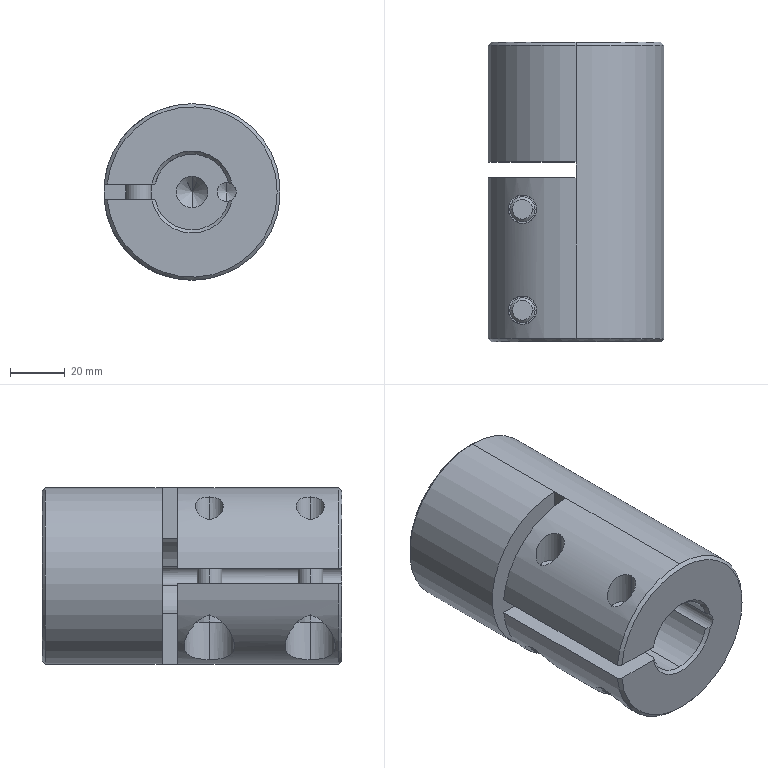Part | SolidWorks | features BaseBody 1 | 1 solid | 90 faces | box 64.615 x 109.615 x 64.615 mm | volume 293786 mm3 | cylinder 34 | plane 31 | cone 25 | commonest cylinder face diameters 10.385 x8 7.482 x6 9.231 x4 16.154 x4 18.462 x4 64.615 x4